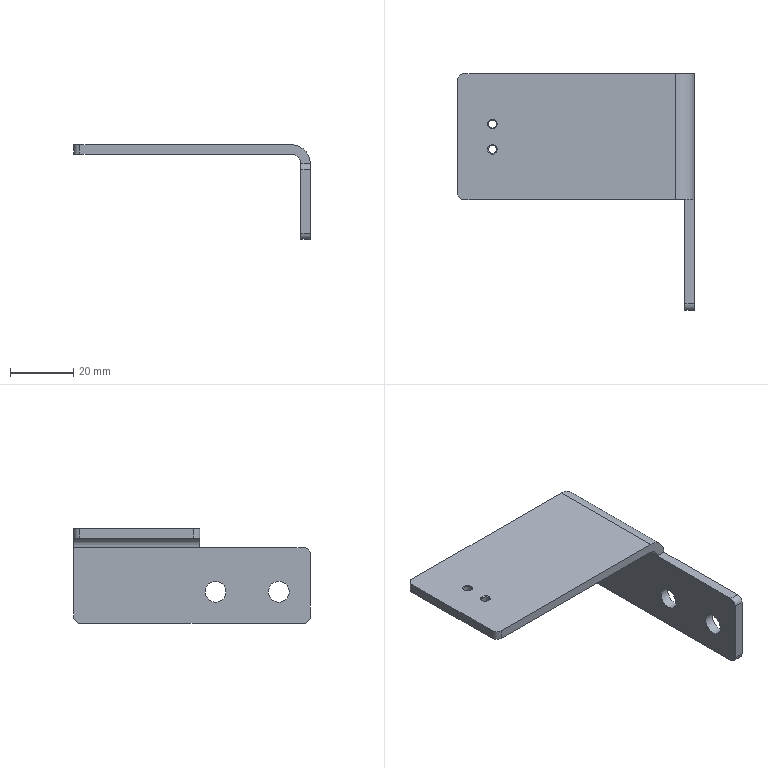Part | NX | features 5003_235_Bracket 2 | 1 solid | 23 faces | box 75 x 75 x 30 mm | volume 14280 mm3 | cylinder 11 | plane 10 | cone 2 | commonest cylinder face diameters 4 x5 2.5 x2 6.6 x2 6 x1 12 x1
STEP:
#1=CARTESIAN_POINT('',(-271.775,-56.6,-22.));
#2=VERTEX_POINT('',#1);
#3=CARTESIAN_POINT('',(-271.775,-20.6,-22.));
#4=VERTEX_POINT('',#3);
#5=CARTESIAN_POINT('',(-271.775,-93.6,-22.));
#6=DIRECTION('',(0.,1.,0.));
#7=VECTOR('',#6,1000.);
#8=LINE('',#5,#7);
#9=EDGE_CURVE('',#2,#4,#8,.T.);
#10=ORIENTED_EDGE('',*,*,#9,.T.);
#11=CARTESIAN_POINT('',(-271.775,-20.6,-25.));
#12=VERTEX_POINT('',#11);
#13=CARTESIAN_POINT('',(-271.775,-20.6,-25.));
#14=DIRECTION('',(0.,0.,1.));
#15=VECTOR('',#14,1000.);
#16=LINE('',#13,#15);
#17=EDGE_CURVE('',#4,#12,#16,.F.);
#18=ORIENTED_EDGE('',*,*,#17,.T.);
#19=CARTESIAN_POINT('',(-271.775,-56.6,-25.));
#20=VERTEX_POINT('',#19);
#21=CARTESIAN_POINT('',(-271.775,-93.6,-25.));
#22=DIRECTION('',(0.,1.,0.));
#23=VECTOR('',#22,1000.);
#24=LINE('',#21,#23);
#25=EDGE_CURVE('',#20,#12,#24,.T.);
#26=ORIENTED_EDGE('',*,*,#25,.F.);
#27=CARTESIAN_POINT('',(-271.775,-56.6,-22.));
#28=DIRECTION('',(0.,0.,-1.));
#29=VECTOR('',#28,1000.);
#30=LINE('',#27,#29);
#31=EDGE_CURVE('',#20,#2,#30,.F.);
#32=ORIENTED_EDGE('',*,*,#31,.T.);
#33=EDGE_LOOP('',(#10,#18,#26,#32));
#34=FACE_BOUND('',#33,.T.);
#35=CARTESIAN_POINT('',(-271.775,-93.6,-22.));
#36=DIRECTION('',(-1.,0.,0.));
#37=DIRECTION('',(0.,-1.,0.));
#38=AXIS2_PLACEMENT_3D('',#35,#36,#37);
#39=PLANE('',#38);
#40=ADVANCED_FACE('',(#34),#39,.T.);
#41=ORIENTED_EDGE('',*,*,#25,.T.);
#42=CARTESIAN_POINT('',(-269.775,-18.6,-25.));
#43=VERTEX_POINT('',#42);
#44=CARTESIAN_POINT('',(-269.775,-20.6,-25.));
#45=DIRECTION('',(0.,0.,-1.));
#46=DIRECTION('',(0.,-1.,0.));
#47=AXIS2_PLACEMENT_3D('',#44,#45,#46);
#48=CIRCLE('',#47,2.);
#49=EDGE_CURVE('',#12,#43,#48,.T.);
#50=ORIENTED_EDGE('',*,*,#49,.T.);
#51=CARTESIAN_POINT('',(-202.775,-18.6,-25.));
#52=VERTEX_POINT('',#51);
#53=CARTESIAN_POINT('',(-202.775,-18.6,-25.));
#54=DIRECTION('',(-1.,0.,0.));
#55=VECTOR('',#54,1000.);
#56=LINE('',#53,#55);
#57=EDGE_CURVE('',#52,#43,#56,.T.);
#58=ORIENTED_EDGE('',*,*,#57,.F.);
#59=CARTESIAN_POINT('',(-202.775,-58.6,-25.));
#60=VERTEX_POINT('',#59);
#61=CARTESIAN_POINT('',(-202.775,-93.6,-25.));
#62=DIRECTION('',(0.,1.,0.));
#63=VECTOR('',#62,1000.);
#64=LINE('',#61,#63);
#65=EDGE_CURVE('',#60,#52,#64,.T.);
#66=ORIENTED_EDGE('',*,*,#65,.F.);
#67=CARTESIAN_POINT('',(-269.775,-58.6,-25.));
#68=VERTEX_POINT('',#67);
#69=CARTESIAN_POINT('',(-196.774,-58.6,-25.));
#70=DIRECTION('',(-1.,0.,0.));
#71=VECTOR('',#70,1000.);
#72=LINE('',#69,#71);
#73=EDGE_CURVE('',#60,#68,#72,.T.);
#74=ORIENTED_EDGE('',*,*,#73,.T.);
#75=CARTESIAN_POINT('',(-269.775,-56.6,-25.));
#76=DIRECTION('',(0.,0.,-1.));
#77=DIRECTION('',(0.,-1.,0.));
#78=AXIS2_PLACEMENT_3D('',#75,#76,#77);
#79=CIRCLE('',#78,2.);
#80=EDGE_CURVE('',#68,#20,#79,.T.);
#81=ORIENTED_EDGE('',*,*,#80,.T.);
#82=EDGE_LOOP('',(#41,#50,#58,#66,#74,#81));
#83=FACE_BOUND('',#82,.T.);
#84=CARTESIAN_POINT('',(-260.775,-35.85,-25.));
#85=VERTEX_POINT('',#84);
#86=CARTESIAN_POINT('',(-260.775,-34.6,-25.));
#87=DIRECTION('',(0.,0.,-1.));
#88=DIRECTION('',(0.,-1.,0.));
#89=AXIS2_PLACEMENT_3D('',#86,#87,#88);
#90=CIRCLE('',#89,1.25);
#91=EDGE_CURVE('',#85,#85,#90,.T.);
#92=ORIENTED_EDGE('',*,*,#91,.F.);
#93=EDGE_LOOP('',(#92));
#94=FACE_BOUND('',#93,.T.);
#95=CARTESIAN_POINT('',(-260.775,-43.85,-25.));
#96=VERTEX_POINT('',#95);
#97=CARTESIAN_POINT('',(-260.775,-42.6,-25.));
#98=DIRECTION('',(0.,0.,-1.));
#99=DIRECTION('',(0.,-1.,0.));
#100=AXIS2_PLACEMENT_3D('',#97,#98,#99);
#101=CIRCLE('',#100,1.25);
#102=EDGE_CURVE('',#96,#96,#101,.T.);
#103=ORIENTED_EDGE('',*,*,#102,.F.);
#104=EDGE_LOOP('',(#103));
#105=FACE_BOUND('',#104,.T.);
#106=CARTESIAN_POINT('',(-202.775,-93.6,-25.));
#107=DIRECTION('',(0.,0.,-1.));
#108=DIRECTION('',(0.,-1.,0.));
#109=AXIS2_PLACEMENT_3D('',#106,#107,#108);
#110=PLANE('',#109);
#111=ADVANCED_FACE('',(#83,#94,#105),#110,.T.);
#112=CARTESIAN_POINT('',(-199.775,-58.6,-28.));
#113=VERTEX_POINT('',#112);
#114=CARTESIAN_POINT('',(-202.775,-58.6,-28.));
#115=DIRECTION('',(0.,1.,0.));
#116=DIRECTION('',(0.,0.,-1.));
#117=AXIS2_PLACEMENT_3D('',#114,#115,#116);
#118=CIRCLE('',#117,3.);
#119=EDGE_CURVE('',#113,#60,#118,.F.);
#120=ORIENTED_EDGE('',*,*,#119,.T.);
#121=ORIENTED_EDGE('',*,*,#65,.T.);
#122=CARTESIAN_POINT('',(-199.775,-18.6,-28.));
#123=VERTEX_POINT('',#122);
#124=CARTESIAN_POINT('',(-202.775,-18.6,-28.));
#125=DIRECTION('',(0.,-1.,0.));
#126=DIRECTION('',(1.,0.,0.));
#127=AXIS2_PLACEMENT_3D('',#124,#125,#126);
#128=CIRCLE('',#127,3.);
#129=EDGE_CURVE('',#123,#52,#128,.T.);
#130=ORIENTED_EDGE('',*,*,#129,.F.);
#131=CARTESIAN_POINT('',(-199.775,-93.6,-28.));
#132=DIRECTION('',(0.,1.,0.));
#133=VECTOR('',#132,1000.);
#134=LINE('',#131,#133);
#135=EDGE_CURVE('',#113,#123,#134,.T.);
#136=ORIENTED_EDGE('',*,*,#135,.F.);
#137=EDGE_LOOP('',(#120,#121,#130,#136));
#138=FACE_BOUND('',#137,.T.);
#139=CARTESIAN_POINT('',(-202.775,-93.6,-28.));
#140=DIRECTION('',(0.,1.,0.));
#141=DIRECTION('',(-1.,0.,0.));
#142=AXIS2_PLACEMENT_3D('',#139,#140,#141);
#143=CYLINDRICAL_SURFACE('',#142,3.);
#144=ADVANCED_FACE('',(#138),#143,.F.);
#145=CARTESIAN_POINT('',(-199.775,-63.6,-38.7));
#146=VERTEX_POINT('',#145);
#147=CARTESIAN_POINT('',(-199.775,-63.6,-42.));
#148=DIRECTION('',(-1.,0.,0.));
#149=DIRECTION('',(0.,0.,1.));
#150=AXIS2_PLACEMENT_3D('',#147,#148,#149);
#151=CIRCLE('',#150,3.3);
#152=EDGE_CURVE('',#146,#146,#151,.T.);
#153=ORIENTED_EDGE('',*,*,#152,.F.);
#154=EDGE_LOOP('',(#153));
#155=FACE_BOUND('',#154,.T.);
#156=CARTESIAN_POINT('',(-199.775,-83.6,-38.7));
#157=VERTEX_POINT('',#156);
#158=CARTESIAN_POINT('',(-199.775,-83.6,-42.));
#159=DIRECTION('',(-1.,0.,0.));
#160=DIRECTION('',(0.,0.,1.));
#161=AXIS2_PLACEMENT_3D('',#158,#159,#160);
#162=CIRCLE('',#161,3.3);
#163=EDGE_CURVE('',#157,#157,#162,.T.);
#164=ORIENTED_EDGE('',*,*,#163,.F.);
#165=EDGE_LOOP('',(#164));
#166=FACE_BOUND('',#165,.T.);
#167=CARTESIAN_POINT('',(-199.775,-93.6,-50.));
#168=VERTEX_POINT('',#167);
#169=CARTESIAN_POINT('',(-199.775,-93.6,-30.));
#170=VERTEX_POINT('',#169);
#171=CARTESIAN_POINT('',(-199.775,-93.6,-52.));
#172=DIRECTION('',(0.,0.,1.));
#173=VECTOR('',#172,1000.);
#174=LINE('',#171,#173);
#175=EDGE_CURVE('',#168,#170,#174,.T.);
#176=ORIENTED_EDGE('',*,*,#175,.T.);
#177=CARTESIAN_POINT('',(-199.775,-91.6,-28.));
#178=VERTEX_POINT('',#177);
#179=CARTESIAN_POINT('',(-199.775,-91.6,-30.));
#180=DIRECTION('',(-1.,0.,0.));
#181=DIRECTION('',(0.,0.,1.));
#182=AXIS2_PLACEMENT_3D('',#179,#180,#181);
#183=CIRCLE('',#182,2.);
#184=EDGE_CURVE('',#170,#178,#183,.T.);
#185=ORIENTED_EDGE('',*,*,#184,.T.);
#186=CARTESIAN_POINT('',(-199.775,-93.6,-28.));
#187=DIRECTION('',(0.,1.,0.));
#188=VECTOR('',#187,1000.);
#189=LINE('',#186,#188);
#190=EDGE_CURVE('',#178,#113,#189,.T.);
#191=ORIENTED_EDGE('',*,*,#190,.T.);
#192=ORIENTED_EDGE('',*,*,#135,.T.);
#193=CARTESIAN_POINT('',(-199.775,-18.6,-50.));
#194=VERTEX_POINT('',#193);
#195=CARTESIAN_POINT('',(-199.775,-18.6,-52.));
#196=DIRECTION('',(0.,0.,1.));
#197=VECTOR('',#196,1000.);
#198=LINE('',#195,#197);
#199=EDGE_CURVE('',#194,#123,#198,.T.);
#200=ORIENTED_EDGE('',*,*,#199,.F.);
#201=CARTESIAN_POINT('',(-199.775,-20.6,-52.));
#202=VERTEX_POINT('',#201);
#203=CARTESIAN_POINT('',(-199.775,-20.6,-50.));
#204=DIRECTION('',(-1.,0.,0.));
#205=DIRECTION('',(0.,0.,1.));
#206=AXIS2_PLACEMENT_3D('',#203,#204,#205);
#207=CIRCLE('',#206,2.);
#208=EDGE_CURVE('',#194,#202,#207,.T.);
#209=ORIENTED_EDGE('',*,*,#208,.T.);
#210=CARTESIAN_POINT('',(-199.775,-91.6,-52.));
#211=VERTEX_POINT('',#210);
#212=CARTESIAN_POINT('',(-199.775,-93.6,-52.));
#213=DIRECTION('',(0.,1.,0.));
#214=VECTOR('',#213,1000.);
#215=LINE('',#212,#214);
#216=EDGE_CURVE('',#211,#202,#215,.T.);
#217=ORIENTED_EDGE('',*,*,#216,.F.);
#218=CARTESIAN_POINT('',(-199.775,-91.6,-50.));
#219=DIRECTION('',(-1.,0.,0.));
#220=DIRECTION('',(0.,0.,1.));
#221=AXIS2_PLACEMENT_3D('',#218,#219,#220);
#222=CIRCLE('',#221,2.);
#223=EDGE_CURVE('',#211,#168,#222,.T.);
#224=ORIENTED_EDGE('',*,*,#223,.T.);
#225=EDGE_LOOP('',(#176,#185,#191,#192,#200,#209,#217,#224));
#226=FACE_BOUND('',#225,.T.);
#227=CARTESIAN_POINT('',(-199.775,-93.6,-52.));
#228=DIRECTION('',(-1.,0.,0.));
#229=DIRECTION('',(0.,0.,1.));
#230=AXIS2_PLACEMENT_3D('',#227,#228,#229);
#231=PLANE('',#230);
#232=ADVANCED_FACE('',(#155,#166,#226),#231,.T.);
#233=CARTESIAN_POINT('',(-196.775,-91.6,-52.));
#234=VERTEX_POINT('',#233);
#235=CARTESIAN_POINT('',(-196.775,-20.6,-52.));
#236=VERTEX_POINT('',#235);
#237=CARTESIAN_POINT('',(-196.775,-93.6,-52.));
#238=DIRECTION('',(0.,1.,0.));
#239=VECTOR('',#238,1000.);
#240=LINE('',#237,#239);
#241=EDGE_CURVE('',#234,#236,#240,.T.);
#242=ORIENTED_EDGE('',*,*,#241,.F.);
#243=CARTESIAN_POINT('',(-196.775,-91.6,-52.));
#244=DIRECTION('',(-1.,0.,0.));
#245=VECTOR('',#244,1000.);
#246=LINE('',#243,#245);
#247=EDGE_CURVE('',#234,#211,#246,.T.);
#248=ORIENTED_EDGE('',*,*,#247,.T.);
#249=ORIENTED_EDGE('',*,*,#216,.T.);
#250=CARTESIAN_POINT('',(-196.775,-20.6,-52.));
#251=DIRECTION('',(-1.,0.,0.));
#252=VECTOR('',#251,1000.);
#253=LINE('',#250,#252);
#254=EDGE_CURVE('',#202,#236,#253,.F.);
#255=ORIENTED_EDGE('',*,*,#254,.T.);
#256=EDGE_LOOP('',(#242,#248,#249,#255));
#257=FACE_BOUND('',#256,.T.);
#258=CARTESIAN_POINT('',(-196.775,-93.6,-52.));
#259=DIRECTION('',(0.,0.,-1.));
#260=DIRECTION('',(0.,-1.,0.));
#261=AXIS2_PLACEMENT_3D('',#258,#259,#260);
#262=PLANE('',#261);
#263=ADVANCED_FACE('',(#257),#262,.T.);
#264=CARTESIAN_POINT('',(-196.775,-63.6,-38.7));
#265=VERTEX_POINT('',#264);
#266=CARTESIAN_POINT('',(-196.775,-63.6,-42.));
#267=DIRECTION('',(-1.,0.,0.));
#268=DIRECTION('',(0.,0.,1.));
#269=AXIS2_PLACEMENT_3D('',#266,#267,#268);
#270=CIRCLE('',#269,3.3);
#271=EDGE_CURVE('',#265,#265,#270,.T.);
#272=ORIENTED_EDGE('',*,*,#271,.T.);
#273=EDGE_LOOP('',(#272));
#274=FACE_BOUND('',#273,.T.);
#275=CARTESIAN_POINT('',(-196.775,-83.6,-38.7));
#276=VERTEX_POINT('',#275);
#277=CARTESIAN_POINT('',(-196.775,-83.6,-42.));
#278=DIRECTION('',(-1.,0.,0.));
#279=DIRECTION('',(0.,0.,1.));
#280=AXIS2_PLACEMENT_3D('',#277,#278,#279);
#281=CIRCLE('',#280,3.3);
#282=EDGE_CURVE('',#276,#276,#281,.T.);
#283=ORIENTED_EDGE('',*,*,#282,.T.);
#284=EDGE_LOOP('',(#283));
#285=FACE_BOUND('',#284,.T.);
#286=CARTESIAN_POINT('',(-196.775,-91.6,-28.));
#287=VERTEX_POINT('',#286);
#288=CARTESIAN_POINT('',(-196.775,-58.6,-28.));
#289=VERTEX_POINT('',#288);
#290=CARTESIAN_POINT('',(-196.775,-93.6,-28.));
#291=DIRECTION('',(0.,1.,0.));
#292=VECTOR('',#291,1000.);
#293=LINE('',#290,#292);
#294=EDGE_CURVE('',#287,#289,#293,.T.);
#295=ORIENTED_EDGE('',*,*,#294,.F.);
#296=CARTESIAN_POINT('',(-196.775,-93.6,-30.));
#297=VERTEX_POINT('',#296);
#298=CARTESIAN_POINT('',(-196.775,-91.6,-30.));
#299=DIRECTION('',(1.,0.,0.));
#300=DIRECTION('',(0.,0.,-1.));
#301=AXIS2_PLACEMENT_3D('',#298,#299,#300);
#302=CIRCLE('',#301,2.);
#303=EDGE_CURVE('',#287,#297,#302,.T.);
#304=ORIENTED_EDGE('',*,*,#303,.T.);
#305=CARTESIAN_POINT('',(-196.775,-93.6,-50.));
#306=VERTEX_POINT('',#305);
#307=CARTESIAN_POINT('',(-196.775,-93.6,-28.));
#308=DIRECTION('',(0.,0.,-1.));
#309=VECTOR('',#308,1000.);
#310=LINE('',#307,#309);
#311=EDGE_CURVE('',#297,#306,#310,.T.);
#312=ORIENTED_EDGE('',*,*,#311,.T.);
#313=CARTESIAN_POINT('',(-196.775,-91.6,-50.));
#314=DIRECTION('',(1.,0.,0.));
#315=DIRECTION('',(0.,0.,-1.));
#316=AXIS2_PLACEMENT_3D('',#313,#314,#315);
#317=CIRCLE('',#316,2.);
#318=EDGE_CURVE('',#306,#234,#317,.T.);
#319=ORIENTED_EDGE('',*,*,#318,.T.);
#320=ORIENTED_EDGE('',*,*,#241,.T.);
#321=CARTESIAN_POINT('',(-196.775,-18.6,-50.));
#322=VERTEX_POINT('',#321);
#323=CARTESIAN_POINT('',(-196.775,-20.6,-50.));
#324=DIRECTION('',(1.,0.,0.));
#325=DIRECTION('',(0.,0.,-1.));
#326=AXIS2_PLACEMENT_3D('',#323,#324,#325);
#327=CIRCLE('',#326,2.);
#328=EDGE_CURVE('',#236,#322,#327,.T.);
#329=ORIENTED_EDGE('',*,*,#328,.T.);
#330=CARTESIAN_POINT('',(-196.775,-18.6,-28.));
#331=VERTEX_POINT('',#330);
#332=CARTESIAN_POINT('',(-196.775,-18.6,-28.));
#333=DIRECTION('',(0.,0.,-1.));
#334=VECTOR('',#333,1000.);
#335=LINE('',#332,#334);
#336=EDGE_CURVE('',#331,#322,#335,.T.);
#337=ORIENTED_EDGE('',*,*,#336,.F.);
#338=CARTESIAN_POINT('',(-196.775,-93.6,-28.));
#339=DIRECTION('',(0.,1.,0.));
#340=VECTOR('',#339,1000.);
#341=LINE('',#338,#340);
#342=EDGE_CURVE('',#289,#331,#341,.T.);
#343=ORIENTED_EDGE('',*,*,#342,.F.);
#344=EDGE_LOOP('',(#295,#304,#312,#319,#320,#329,#337,#343));
#345=FACE_BOUND('',#344,.T.);
#346=CARTESIAN_POINT('',(-196.775,-93.6,-28.));
#347=DIRECTION('',(1.,0.,0.));
#348=DIRECTION('',(0.,0.,-1.));
#349=AXIS2_PLACEMENT_3D('',#346,#347,#348);
#350=PLANE('',#349);
#351=ADVANCED_FACE('',(#274,#285,#345),#350,.T.);
#352=CARTESIAN_POINT('',(-202.775,-58.6,-22.));
#353=VERTEX_POINT('',#352);
#354=CARTESIAN_POINT('',(-202.775,-58.6,-28.));
#355=DIRECTION('',(0.,1.,0.));
#356=DIRECTION('',(0.,0.,-1.));
#357=AXIS2_PLACEMENT_3D('',#354,#355,#356);
#358=CIRCLE('',#357,6.);
#359=EDGE_CURVE('',#353,#289,#358,.T.);
#360=ORIENTED_EDGE('',*,*,#359,.T.);
#361=ORIENTED_EDGE('',*,*,#342,.T.);
#362=CARTESIAN_POINT('',(-202.775,-18.6,-22.));
#363=VERTEX_POINT('',#362);
#364=CARTESIAN_POINT('',(-202.775,-18.6,-28.));
#365=DIRECTION('',(0.,1.,0.));
#366=DIRECTION('',(1.,0.,0.));
#367=AXIS2_PLACEMENT_3D('',#364,#365,#366);
#368=CIRCLE('',#367,6.);
#369=EDGE_CURVE('',#363,#331,#368,.T.);
#370=ORIENTED_EDGE('',*,*,#369,.F.);
#371=CARTESIAN_POINT('',(-202.775,-93.6,-22.));
#372=DIRECTION('',(0.,1.,0.));
#373=VECTOR('',#372,1000.);
#374=LINE('',#371,#373);
#375=EDGE_CURVE('',#353,#363,#374,.T.);
#376=ORIENTED_EDGE('',*,*,#375,.F.);
#377=EDGE_LOOP('',(#360,#361,#370,#376));
#378=FACE_BOUND('',#377,.T.);
#379=CARTESIAN_POINT('',(-202.775,-93.6,-28.));
#380=DIRECTION('',(0.,1.,0.));
#381=DIRECTION('',(-1.,0.,0.));
#382=AXIS2_PLACEMENT_3D('',#379,#380,#381);
#383=CYLINDRICAL_SURFACE('',#382,6.);
#384=ADVANCED_FACE('',(#378),#383,.T.);
#385=CARTESIAN_POINT('',(-269.775,-18.6,-22.));
#386=VERTEX_POINT('',#385);
#387=CARTESIAN_POINT('',(-202.775,-18.6,-22.));
#388=DIRECTION('',(1.,0.,0.));
#389=VECTOR('',#388,1000.);
#390=LINE('',#387,#389);
#391=EDGE_CURVE('',#386,#363,#390,.T.);
#392=ORIENTED_EDGE('',*,*,#391,.F.);
#393=CARTESIAN_POINT('',(-269.775,-20.6,-22.));
#394=DIRECTION('',(0.,0.,1.));
#395=DIRECTION('',(0.,1.,0.));
#396=AXIS2_PLACEMENT_3D('',#393,#394,#395);
#397=CIRCLE('',#396,2.);
#398=EDGE_CURVE('',#386,#4,#397,.T.);
#399=ORIENTED_EDGE('',*,*,#398,.T.);
#400=ORIENTED_EDGE('',*,*,#9,.F.);
#401=CARTESIAN_POINT('',(-269.775,-58.6,-22.));
#402=VERTEX_POINT('',#401);
#403=CARTESIAN_POINT('',(-269.775,-56.6,-22.));
#404=DIRECTION('',(0.,0.,1.));
#405=DIRECTION('',(0.,1.,0.));
#406=AXIS2_PLACEMENT_3D('',#403,#404,#405);
#407=CIRCLE('',#406,2.);
#408=EDGE_CURVE('',#2,#402,#407,.T.);
#409=ORIENTED_EDGE('',*,*,#408,.T.);
#410=CARTESIAN_POINT('',(-196.774,-58.6,-22.));
#411=DIRECTION('',(-1.,0.,0.));
#412=VECTOR('',#411,1000.);
#413=LINE('',#410,#412);
#414=EDGE_CURVE('',#353,#402,#413,.T.);
#415=ORIENTED_EDGE('',*,*,#414,.F.);
#416=ORIENTED_EDGE('',*,*,#375,.T.);
#417=EDGE_LOOP('',(#392,#399,#400,#409,#415,#416));
#418=FACE_BOUND('',#417,.T.);
#419=CARTESIAN_POINT('',(-260.775,-33.075,-22.));
#420=VERTEX_POINT('',#419);
#421=CARTESIAN_POINT('',(-260.775,-34.6,-22.));
#422=DIRECTION('',(0.,0.,1.));
#423=DIRECTION('',(0.,1.,0.));
#424=AXIS2_PLACEMENT_3D('',#421,#422,#423);
#425=CIRCLE('',#424,1.525);
#426=EDGE_CURVE('',#420,#420,#425,.T.);
#427=ORIENTED_EDGE('',*,*,#426,.F.);
#428=EDGE_LOOP('',(#427));
#429=FACE_BOUND('',#428,.T.);
#430=CARTESIAN_POINT('',(-260.775,-41.075,-22.));
#431=VERTEX_POINT('',#430);
#432=CARTESIAN_POINT('',(-260.775,-42.6,-22.));
#433=DIRECTION('',(0.,0.,1.));
#434=DIRECTION('',(0.,1.,0.));
#435=AXIS2_PLACEMENT_3D('',#432,#433,#434);
#436=CIRCLE('',#435,1.525);
#437=EDGE_CURVE('',#431,#431,#436,.T.);
#438=ORIENTED_EDGE('',*,*,#437,.F.);
#439=EDGE_LOOP('',(#438));
#440=FACE_BOUND('',#439,.T.);
#441=CARTESIAN_POINT('',(-202.775,-93.6,-22.));
#442=DIRECTION('',(0.,0.,1.));
#443=DIRECTION('',(0.,1.,0.));
#444=AXIS2_PLACEMENT_3D('',#441,#442,#443);
#445=PLANE('',#444);
#446=ADVANCED_FACE('',(#418,#429,#440),#445,.T.);
#447=ORIENTED_EDGE('',*,*,#311,.F.);
#448=CARTESIAN_POINT('',(-199.775,-93.6,-30.));
#449=DIRECTION('',(-1.,0.,0.));
#450=VECTOR('',#449,1000.);
#451=LINE('',#448,#450);
#452=EDGE_CURVE('',#297,#170,#451,.T.);
#453=ORIENTED_EDGE('',*,*,#452,.T.);
#454=ORIENTED_EDGE('',*,*,#175,.F.);
#455=CARTESIAN_POINT('',(-202.775,-93.6,-50.));
#456=DIRECTION('',(-1.,0.,0.));
#457=VECTOR('',#456,1000.);
#458=LINE('',#455,#457);
#459=EDGE_CURVE('',#168,#306,#458,.F.);
#460=ORIENTED_EDGE('',*,*,#459,.T.);
#461=EDGE_LOOP('',(#447,#453,#454,#460));
#462=FACE_BOUND('',#461,.T.);
#463=CARTESIAN_POINT('',(-202.775,-93.6,-28.));
#464=DIRECTION('',(0.,-1.,0.));
#465=DIRECTION('',(1.,0.,0.));
#466=AXIS2_PLACEMENT_3D('',#463,#464,#465);
#467=PLANE('',#466);
#468=ADVANCED_FACE('',(#462),#467,.T.);
#469=ORIENTED_EDGE('',*,*,#336,.T.);
#470=CARTESIAN_POINT('',(-199.775,-18.6,-50.));
#471=DIRECTION('',(-1.,0.,0.));
#472=VECTOR('',#471,1000.);
#473=LINE('',#470,#472);
#474=EDGE_CURVE('',#322,#194,#473,.T.);
#475=ORIENTED_EDGE('',*,*,#474,.T.);
#476=ORIENTED_EDGE('',*,*,#199,.T.);
#477=ORIENTED_EDGE('',*,*,#129,.T.);
#478=ORIENTED_EDGE('',*,*,#57,.T.);
#479=CARTESIAN_POINT('',(-269.775,-18.6,-22.));
#480=DIRECTION('',(0.,0.,1.));
#481=VECTOR('',#480,1000.);
#482=LINE('',#479,#481);
#483=EDGE_CURVE('',#43,#386,#482,.T.);
#484=ORIENTED_EDGE('',*,*,#483,.T.);
#485=ORIENTED_EDGE('',*,*,#391,.T.);
#486=ORIENTED_EDGE('',*,*,#369,.T.);
#487=EDGE_LOOP('',(#469,#475,#476,#477,#478,#484,#485,#486));
#488=FACE_BOUND('',#487,.T.);
#489=CARTESIAN_POINT('',(-202.775,-18.6,-28.));
#490=DIRECTION('',(0.,-1.,0.));
#491=DIRECTION('',(1.,0.,0.));
#492=AXIS2_PLACEMENT_3D('',#489,#490,#491);
#493=PLANE('',#492);
#494=ADVANCED_FACE('',(#488),#493,.F.);
#495=ORIENTED_EDGE('',*,*,#282,.F.);
#496=EDGE_LOOP('',(#495));
#497=FACE_BOUND('',#496,.T.);
#498=ORIENTED_EDGE('',*,*,#163,.T.);
#499=EDGE_LOOP('',(#498));
#500=FACE_BOUND('',#499,.T.);
#501=CARTESIAN_POINT('',(-196.775,-83.6,-42.));
#502=DIRECTION('',(-1.,0.,0.));
#503=DIRECTION('',(0.,0.,1.));
#504=AXIS2_PLACEMENT_3D('',#501,#502,#503);
#505=CYLINDRICAL_SURFACE('',#504,3.3);
#506=ADVANCED_FACE('',(#497,#500),#505,.F.);
#507=ORIENTED_EDGE('',*,*,#271,.F.);
#508=EDGE_LOOP('',(#507));
#509=FACE_BOUND('',#508,.T.);
#510=ORIENTED_EDGE('',*,*,#152,.T.);
#511=EDGE_LOOP('',(#510));
#512=FACE_BOUND('',#511,.T.);
#513=CARTESIAN_POINT('',(-196.775,-63.6,-42.));
#514=DIRECTION('',(-1.,0.,0.));
#515=DIRECTION('',(0.,0.,1.));
#516=AXIS2_PLACEMENT_3D('',#513,#514,#515);
#517=CYLINDRICAL_SURFACE('',#516,3.3);
#518=ADVANCED_FACE('',(#509,#512),#517,.F.);
#519=ORIENTED_EDGE('',*,*,#102,.T.);
#520=EDGE_LOOP('',(#519));
#521=FACE_BOUND('',#520,.T.);
#522=CARTESIAN_POINT('',(-260.775,-41.35,-22.275));
#523=VERTEX_POINT('',#522);
#524=CARTESIAN_POINT('',(-260.775,-42.6,-22.275));
#525=DIRECTION('',(0.,0.,1.));
#526=DIRECTION('',(0.,1.,0.));
#527=AXIS2_PLACEMENT_3D('',#524,#525,#526);
#528=CIRCLE('',#527,1.25);
#529=EDGE_CURVE('',#523,#523,#528,.T.);
#530=ORIENTED_EDGE('',*,*,#529,.T.);
#531=EDGE_LOOP('',(#530));
#532=FACE_BOUND('',#531,.T.);
#533=CARTESIAN_POINT('',(-260.775,-42.6,-22.));
#534=DIRECTION('',(0.,0.,1.));
#535=DIRECTION('',(0.,1.,0.));
#536=AXIS2_PLACEMENT_3D('',#533,#534,#535);
#537=CYLINDRICAL_SURFACE('',#536,1.25);
#538=ADVANCED_FACE('',(#521,#532),#537,.F.);
#539=ORIENTED_EDGE('',*,*,#529,.F.);
#540=EDGE_LOOP('',(#539));
#541=FACE_BOUND('',#540,.T.);
#542=ORIENTED_EDGE('',*,*,#437,.T.);
#543=EDGE_LOOP('',(#542));
#544=FACE_BOUND('',#543,.T.);
#545=CARTESIAN_POINT('',(-260.775,-42.6,-22.));
#546=DIRECTION('',(0.,0.,1.));
#547=DIRECTION('',(0.,1.,0.));
#548=AXIS2_PLACEMENT_3D('',#545,#546,#547);
#549=CONICAL_SURFACE('',#548,1.525,0.7854);
#550=ADVANCED_FACE('',(#541,#544),#549,.F.);
#551=ORIENTED_EDGE('',*,*,#91,.T.);
#552=EDGE_LOOP('',(#551));
#553=FACE_BOUND('',#552,.T.);
#554=CARTESIAN_POINT('',(-260.775,-33.35,-22.275));
#555=VERTEX_POINT('',#554);
#556=CARTESIAN_POINT('',(-260.775,-34.6,-22.275));
#557=DIRECTION('',(0.,0.,1.));
#558=DIRECTION('',(0.,1.,0.));
#559=AXIS2_PLACEMENT_3D('',#556,#557,#558);
#560=CIRCLE('',#559,1.25);
#561=EDGE_CURVE('',#555,#555,#560,.T.);
#562=ORIENTED_EDGE('',*,*,#561,.T.);
#563=EDGE_LOOP('',(#562));
#564=FACE_BOUND('',#563,.T.);
#565=CARTESIAN_POINT('',(-260.775,-34.6,-22.));
#566=DIRECTION('',(0.,0.,1.));
#567=DIRECTION('',(0.,1.,0.));
#568=AXIS2_PLACEMENT_3D('',#565,#566,#567);
#569=CYLINDRICAL_SURFACE('',#568,1.25);
#570=ADVANCED_FACE('',(#553,#564),#569,.F.);
#571=ORIENTED_EDGE('',*,*,#561,.F.);
#572=EDGE_LOOP('',(#571));
#573=FACE_BOUND('',#572,.T.);
#574=ORIENTED_EDGE('',*,*,#426,.T.);
#575=EDGE_LOOP('',(#574));
#576=FACE_BOUND('',#575,.T.);
#577=CARTESIAN_POINT('',(-260.775,-34.6,-22.));
#578=DIRECTION('',(0.,0.,1.));
#579=DIRECTION('',(0.,1.,0.));
#580=AXIS2_PLACEMENT_3D('',#577,#578,#579);
#581=CONICAL_SURFACE('',#580,1.525,0.7854);
#582=ADVANCED_FACE('',(#573,#576),#581,.F.);
#583=ORIENTED_EDGE('',*,*,#414,.T.);
#584=CARTESIAN_POINT('',(-269.775,-58.6,-25.));
#585=DIRECTION('',(0.,0.,-1.));
#586=VECTOR('',#585,1000.);
#587=LINE('',#584,#586);
#588=EDGE_CURVE('',#402,#68,#587,.T.);
#589=ORIENTED_EDGE('',*,*,#588,.T.);
#590=ORIENTED_EDGE('',*,*,#73,.F.);
#591=ORIENTED_EDGE('',*,*,#119,.F.);
#592=CARTESIAN_POINT('',(-196.774,-58.6,-28.));
#593=DIRECTION('',(-1.,0.,0.));
#594=VECTOR('',#593,1000.);
#595=LINE('',#592,#594);
#596=EDGE_CURVE('',#289,#113,#595,.T.);
#597=ORIENTED_EDGE('',*,*,#596,.F.);
#598=ORIENTED_EDGE('',*,*,#359,.F.);
#599=EDGE_LOOP('',(#583,#589,#590,#591,#597,#598));
#600=FACE_BOUND('',#599,.T.);
#601=CARTESIAN_POINT('',(-196.774,-58.6,-22.));
#602=DIRECTION('',(0.,1.,0.));
#603=DIRECTION('',(0.,0.,-1.));
#604=AXIS2_PLACEMENT_3D('',#601,#602,#603);
#605=PLANE('',#604);
#606=ADVANCED_FACE('',(#600),#605,.F.);
#607=ORIENTED_EDGE('',*,*,#190,.F.);
#608=CARTESIAN_POINT('',(-196.775,-91.6,-28.));
#609=DIRECTION('',(-1.,0.,0.));
#610=VECTOR('',#609,1000.);
#611=LINE('',#608,#610);
#612=EDGE_CURVE('',#178,#287,#611,.F.);
#613=ORIENTED_EDGE('',*,*,#612,.T.);
#614=ORIENTED_EDGE('',*,*,#294,.T.);
#615=ORIENTED_EDGE('',*,*,#596,.T.);
#616=EDGE_LOOP('',(#607,#613,#614,#615));
#617=FACE_BOUND('',#616,.T.);
#618=CARTESIAN_POINT('',(-196.774,-58.6,-28.));
#619=DIRECTION('',(0.,0.,-1.));
#620=DIRECTION('',(0.,-1.,0.));
#621=AXIS2_PLACEMENT_3D('',#618,#619,#620);
#622=PLANE('',#621);
#623=ADVANCED_FACE('',(#617),#622,.F.);
#624=ORIENTED_EDGE('',*,*,#303,.F.);
#625=ORIENTED_EDGE('',*,*,#612,.F.);
#626=ORIENTED_EDGE('',*,*,#184,.F.);
#627=ORIENTED_EDGE('',*,*,#452,.F.);
#628=EDGE_LOOP('',(#624,#625,#626,#627));
#629=FACE_BOUND('',#628,.T.);
#630=CARTESIAN_POINT('',(-202.775,-91.6,-30.));
#631=DIRECTION('',(1.,0.,0.));
#632=DIRECTION('',(0.,1.,0.));
#633=AXIS2_PLACEMENT_3D('',#630,#631,#632);
#634=CYLINDRICAL_SURFACE('',#633,2.);
#635=ADVANCED_FACE('',(#629),#634,.T.);
#636=ORIENTED_EDGE('',*,*,#318,.F.);
#637=ORIENTED_EDGE('',*,*,#459,.F.);
#638=ORIENTED_EDGE('',*,*,#223,.F.);
#639=ORIENTED_EDGE('',*,*,#247,.F.);
#640=EDGE_LOOP('',(#636,#637,#638,#639));
#641=FACE_BOUND('',#640,.T.);
#642=CARTESIAN_POINT('',(-196.775,-91.6,-50.));
#643=DIRECTION('',(-1.,0.,0.));
#644=DIRECTION('',(0.,-1.,0.));
#645=AXIS2_PLACEMENT_3D('',#642,#643,#644);
#646=CYLINDRICAL_SURFACE('',#645,2.);
#647=ADVANCED_FACE('',(#641),#646,.T.);
#648=ORIENTED_EDGE('',*,*,#328,.F.);
#649=ORIENTED_EDGE('',*,*,#254,.F.);
#650=ORIENTED_EDGE('',*,*,#208,.F.);
#651=ORIENTED_EDGE('',*,*,#474,.F.);
#652=EDGE_LOOP('',(#648,#649,#650,#651));
#653=FACE_BOUND('',#652,.T.);
#654=CARTESIAN_POINT('',(-202.775,-20.6,-50.));
#655=DIRECTION('',(1.,0.,0.));
#656=DIRECTION('',(0.,1.,0.));
#657=AXIS2_PLACEMENT_3D('',#654,#655,#656);
#658=CYLINDRICAL_SURFACE('',#657,2.);
#659=ADVANCED_FACE('',(#653),#658,.T.);
#660=ORIENTED_EDGE('',*,*,#49,.F.);
#661=ORIENTED_EDGE('',*,*,#17,.F.);
#662=ORIENTED_EDGE('',*,*,#398,.F.);
#663=ORIENTED_EDGE('',*,*,#483,.F.);
#664=EDGE_LOOP('',(#660,#661,#662,#663));
#665=FACE_BOUND('',#664,.T.);
#666=CARTESIAN_POINT('',(-269.775,-20.6,-28.));
#667=DIRECTION('',(0.,0.,-1.));
#668=DIRECTION('',(0.,-1.,0.));
#669=AXIS2_PLACEMENT_3D('',#666,#667,#668);
#670=CYLINDRICAL_SURFACE('',#669,2.);
#671=ADVANCED_FACE('',(#665),#670,.T.);
#672=ORIENTED_EDGE('',*,*,#408,.F.);
#673=ORIENTED_EDGE('',*,*,#31,.F.);
#674=ORIENTED_EDGE('',*,*,#80,.F.);
#675=ORIENTED_EDGE('',*,*,#588,.F.);
#676=EDGE_LOOP('',(#672,#673,#674,#675));
#677=FACE_BOUND('',#676,.T.);
#678=CARTESIAN_POINT('',(-269.775,-56.6,-22.));
#679=DIRECTION('',(0.,0.,1.));
#680=DIRECTION('',(0.,1.,0.));
#681=AXIS2_PLACEMENT_3D('',#678,#679,#680);
#682=CYLINDRICAL_SURFACE('',#681,2.);
#683=ADVANCED_FACE('',(#677),#682,.T.);
#684=CLOSED_SHELL('',(#40,#111,#144,#232,#263,#351,#384,#446,#468,#494,#506,#518,#538,#550,#570,#582,#606,#623,#635,#647,#659,#671,#683));
#685=MANIFOLD_SOLID_BREP('',#684);
#686=(LENGTH_UNIT()NAMED_UNIT(*)SI_UNIT(.MILLI.,.METRE.));
#687=UNCERTAINTY_MEASURE_WITH_UNIT(LENGTH_MEASURE(0.00001),#686,'','');
#688=(NAMED_UNIT(*)PLANE_ANGLE_UNIT()SI_UNIT($,.RADIAN.));
#689=(NAMED_UNIT(*)SI_UNIT($,.STERADIAN.)SOLID_ANGLE_UNIT());
#690=(GEOMETRIC_REPRESENTATION_CONTEXT(3)GLOBAL_UNCERTAINTY_ASSIGNED_CONTEXT((#687))GLOBAL_UNIT_ASSIGNED_CONTEXT((#686,#688,#689))REPRESENTATION_CONTEXT('',''));
#691=ADVANCED_BREP_SHAPE_REPRESENTATION('',(#685),#690);